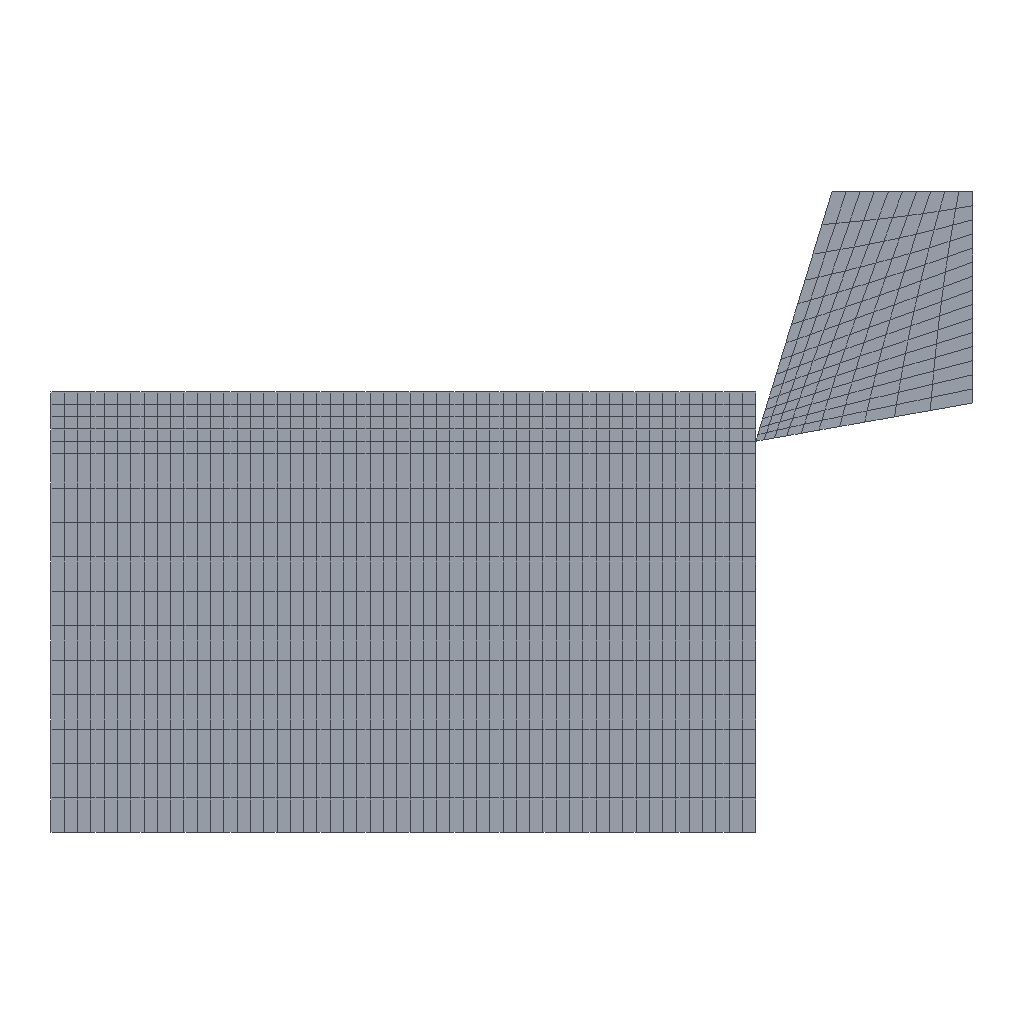Simulation study | abaqus
Set-up summary:
category,name,step,type,value,unit,region
solver,abaqus
solver,version,,,Abaqus/Explicit 3DEXPERIENCE R2017x
units,not stated in the deck,,not stated
analysis,deck,,dynamic temperature-displacement,dynamic temperature-displacement
load_step,Step-1,Step-1,dynamic temperature-displacement
load_step,requested,,,1
mesh,nodes,,,1094
mesh,elements,,,998
element_type,CPE4RT,,plane,998
load,load commands in deck,,count,1
bc,support commands in deck,,count,4
material,CFRP,,in results
material,CFRP-COPY,,in results
material,TOOL,,in results
check,setup vs results,,match,"per instance, exact: element labels, types and connectivity; labels of the nodes the elements use; coordinates of those nodes at SINGLE_PRECISION in 2 of 2 instance(s)"
Abaqus input file, long lists of numbers shortened:
*Heading
** Job name: Job-a Model name: [REDACTED]
** Generated by: Abaqus/CAE 2017
*Preprint, echo=NO, model=NO, history=NO, contact=NO
**
** PARTS
**
*Part, name=TOOL
*Node
      1,           0.,           0.
      2,  0.9701,  0.1711
** (174 more lines like these left out)
*Element, type=CPE4RT
  1,   1,   2,  13,  12
  2,   2,   3,  14,  13
** (148 more lines like these left out)
*Nset, nset=SET-1, generate
   1,  176,    1
*Elset, elset=SET-1, generate
   1,  150,    1
** Section: Section-1-SET-1
*Solid Section, elset=SET-1, material=TOOL
,
*End Part
**
*Part, name=WORK
*Node
      1,          80.,          -7.
      2,           0.,          -7.
** (916 more lines like these left out)
*Element, type=CPE4RT
  1,   1,   7, 191, 130
  2,   7,   8, 192, 191
** (846 more lines like these left out)
*Nset, nset=SET-6, generate
   1,  918,    1
*Elset, elset=SET-6, generate
   1,  848,    1
*Elset, elset=Set-3, generate
 584,  848,    1
*Elset, elset=Set-4, generate
   1,  583,    1
*Orientation, name=Ori-1
1., 0., 0., 0., 1., 0.
3, 0.
** Section: no
*Solid Section, elset=Set-4, orientation=Ori-1, material=CFRP-Copy
,
** Section: Section-2-SET-6
*Solid Section, elset=Set-3, orientation=Ori-1, material=CFRP
,
*End Part
**
**
** ASSEMBLY
**
*Assembly, name=Assembly
**
*Instance, name=TOOL-1, part=TOOL
         80.,         -5.6,           0.
*End Instance
**
*Instance, name=WORK-1, part=WORK
*End Instance
**
*Node
      1,   104.667,    21.85
*Nset, nset=B_SET-2, instance=TOOL-1, generate
   1,  176,    1
*Elset, elset=B_SET-2, instance=TOOL-1, generate
   1,  150,    1
*Nset, nset=SET-1, instance=WORK-1
   3,   4,  69,  70,  71,  72,  73,  74,  75,  76,  77,  78,  79,  80,  81,  82
  83,  84,  85,  86,  87,  88,  89,  90,  91,  92,  93,  94,  95,  96,  97,  98
** (2 more lines like these left out)
*Elset, elset=SET-1, instance=WORK-1, generate
 531,  583,    1
*Nset, nset=SET-5
 1,
*Nset, nset=SET-6
 1,
*Nset, nset=SET-7, instance=WORK-1
   3,   4,  69,  70,  71,  72,  73,  74,  75,  76,  77,  78,  79,  80,  81,  82
  83,  84,  85,  86,  87,  88,  89,  90,  91,  92,  93,  94,  95,  96,  97,  98
** (2 more lines like these left out)
*Elset, elset=SET-7, instance=WORK-1, generate
 531,  583,    1
*Nset, nset=S_SET-4, instance=WORK-1
   5,   6, 135, 136, 137, 138, 139, 140, 141, 142, 143, 144, 145, 146, 147, 148
 149, 150, 151, 152, 153, 154, 155, 156, 157, 158, 159, 160, 161, 162, 163, 164
** (2 more lines like these left out)
*Elset, elset=S_SET-4, instance=WORK-1, generate
 796,  848,    1
*Nset, nset=S_SET-8, instance=WORK-1
   1,   2,   5,   6,   7,   8,   9,  10,  11,  12,  13,  14,  15,  16,  17,  18
  19,  20,  21,  22,  23,  24,  25,  26,  27,  28,  29,  30,  31,  32,  33,  34
** (19 more lines like these left out)
*Elset, elset=S_SET-8, instance=WORK-1, generate
 584,  848,    1
*Nset, nset=Set-13, instance=WORK-1
   2,   3,   4,   6,  59,  60,  61,  62,  63,  64,  65,  66,  67,  68,  69,  70
  71,  72,  73,  74,  75,  76,  77,  78,  79,  80,  81,  82,  83,  84,  85,  86
** (6 more lines like these left out)
*Nset, nset=S_SET-8_CNS_, internal, instance=WORK-1
   1,   2,   5,   6,   7,   8,   9,  10,  11,  12,  13,  14,  15,  16,  17,  18
  19,  20,  21,  22,  23,  24,  25,  26,  27,  28,  29,  30,  31,  32,  33,  34
** (19 more lines like these left out)
*Elset, elset=_M_SURF-1_S1, internal, instance=TOOL-1, generate
  1,  10,   1
*Elset, elset=_M_SURF-1_S4, internal, instance=TOOL-1, generate
   1,  141,   10
*Nset, nset=_PICKEDSET9, internal
 1,
*Nset, nset=_PickedSet23, internal
 1,
*Elset, elset=_M_SURF-1_S1_1, internal, instance=TOOL-1, generate
  1,  10,   1
*Elset, elset=_M_SURF-1_S4_1, internal, instance=TOOL-1, generate
   1,  141,   10
*Surface, type=ELEMENT, name=M_SURF-1
_M_SURF-1_S1_1, S1
_M_SURF-1_S4_1, S4
*Surface, type=NODE, name=S_SET-8_CNS__CNS_, internal
S_SET-8_CNS_, 1.
** Constraint: RigidBody-1
*Rigid Body, ref node=_PickedSet23, elset=B_SET-2
*End Assembly
*Amplitude, name=AMP-1
             0.,              0.,              5.,              1.
**
** MATERIALS
**
*Material, name=CFRP
*Conductivity
 0.5,
*Density
 2e-09,
*Depvar, delete=5
     17,
*Expansion
 8.5e-06,
*Specific Heat
 8e+08,
*User Material, constants=27
2900., 1500., 2500.,   0.3,   0.4,   0.3,  500.,  500.
  500., 1e-09,   30.,   30.,   30.,   30.,    0.,    0.
 1500.,  958.,  958.,  900.,  985.,  985.,    0.,    0.
 1276., 1250., 1250.
*Material, name=CFRP-Copy
*Conductivity
 0.5,
*Density
 2e-09,
*Elastic, type=ENGINEERING CONSTANTS
54000.,54000.,54000.,  0.25,  0.35,  0.35,16000.,24000.
24000.,
*Expansion
 8.5e-06,
*Specific Heat
 8e+08,
*Material, name=TOOL
*Conductivity
45.,
*Density
 7.8e-09,
*Elastic
210000., 0.3
*Specific Heat
 4.6e+08,
**
** INTERACTION PROPERTIES
**
*Surface Interaction, name=INTPROP-1
*Friction
 0.2,
*Surface Behavior, pressure-overclosure=HARD
*Gap Conductance
 0.1,    0.
  0., 0.001
** ----------------------------------------------------------------
**
** STEP: Step-1
**
*Step, name=Step-1, nlgeom=YES
*Dynamic Temperature-displacement, Explicit
, 5.
*Bulk Viscosity
0.06, 1.2
** Mass Scaling: Semi-Automatic
**               Whole Model
*Fixed Mass Scaling, factor=500.
**
** BOUNDARY CONDITIONS
**
** Name: Disp-BC-1 Type: 对称/反对称/完全固定
*Boundary
Set-13, ENCASTRE
** Name: Disp-BC-2 Type: 位移/转角
*Boundary, amplitude=AMP-1
SET-6, 1, 1, -80.
** Name: Disp-BC-3 Type: 位移/转角
*Boundary, amplitude=AMP-1
SET-6, 2, 2
** Name: Disp-BC-4 Type: 位移/转角
*Boundary, amplitude=AMP-1
SET-6, 6, 6
**
** INTERACTIONS
**
** Interaction: INT-1-1
*Contact Pair, interaction=INTPROP-1, mechanical constraint=KINEMATIC, cpset=INT-1-1
M_SURF-1, S_SET-8_CNS__CNS_
**
** OUTPUT REQUESTS
**
*Restart, write, number interval=1, time marks=NO
**
** FIELD OUTPUT: F-Output-1
**
*Output, field, number interval=50
*Node Output
CF, NT, RF, RM, RT, U, V
*Element Output, directions=YES
E, FV, HFL, LE, MISES, MISESMAX, PE, PEEQ, PEEQMAX, PEEQT, PEEQVAVG, PEMAG, PEVAVG, S, SDV, SSAVG
STATUS, SVAVG, TEMP
*Contact Output
CDISP, CSTRESS
**
** HISTORY OUTPUT: H-Output-1
**
*Output, history, time interval=0.0005
*Node Output, nset=SET-5
RF1, RF2
*End Step
Results summary:
result,step,Step-1,partial,increments=123636 time=0.5791/5.0
result,analysis,,,"dynamic temperature-displacement, explict"
result,last_loadstep,,,1
result,primary field,,,"U, NT11"
result,reaction total,,FX,0.198,model units
result,reaction total,,FY,-0.05518,model units
result,reaction total,,FZ,0.0,model units